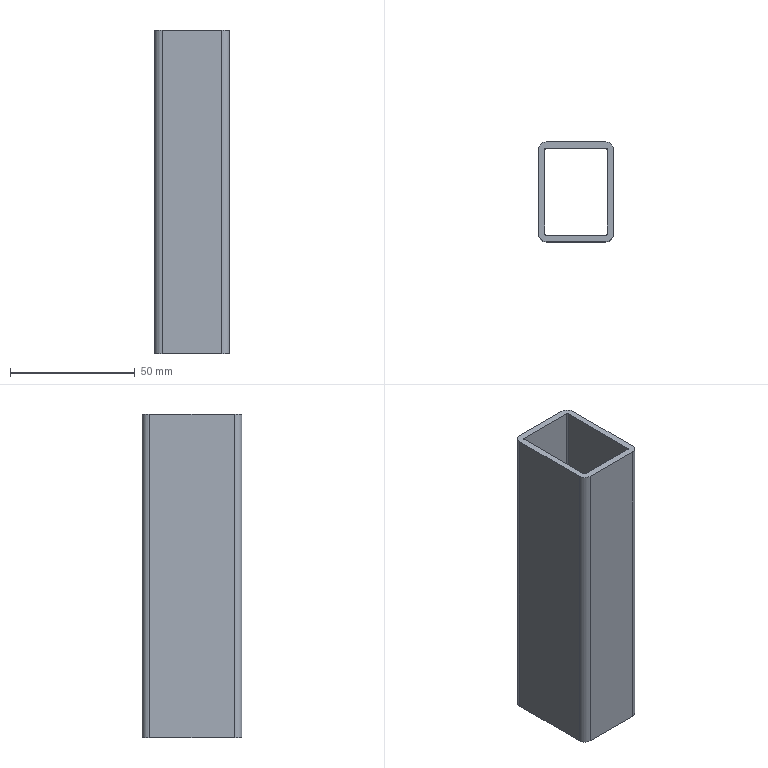Part | SolidWorks | features BaseBody 1 | 1 solid | 18 faces | box 30 x 40 x 130 mm | volume 41274 mm3 | plane 10 | cylinder 8 | commonest cylinder face diameters 1 x4 6 x4
STEP:
#1=CARTESIAN_POINT('',(12.,17.5,-65.));
#2=VERTEX_POINT('',#1);
#3=CARTESIAN_POINT('',(-12.,17.5,-65.));
#4=VERTEX_POINT('',#3);
#5=CARTESIAN_POINT('',(-12.,17.5,-65.));
#6=DIRECTION('',(-1.,0.,0.));
#7=VECTOR('',#6,1000.);
#8=LINE('',#5,#7);
#9=EDGE_CURVE('',#2,#4,#8,.T.);
#10=ORIENTED_EDGE('',*,*,#9,.F.);
#11=CARTESIAN_POINT('',(12.,17.5,65.));
#12=VERTEX_POINT('',#11);
#13=CARTESIAN_POINT('',(12.,17.5,65.));
#14=DIRECTION('',(0.,0.,-1.));
#15=VECTOR('',#14,1000.);
#16=LINE('',#13,#15);
#17=EDGE_CURVE('',#12,#2,#16,.T.);
#18=ORIENTED_EDGE('',*,*,#17,.F.);
#19=CARTESIAN_POINT('',(-12.,17.5,65.));
#20=VERTEX_POINT('',#19);
#21=CARTESIAN_POINT('',(-12.,17.5,65.));
#22=DIRECTION('',(-1.,0.,0.));
#23=VECTOR('',#22,1000.);
#24=LINE('',#21,#23);
#25=EDGE_CURVE('',#12,#20,#24,.T.);
#26=ORIENTED_EDGE('',*,*,#25,.T.);
#27=CARTESIAN_POINT('',(-12.,17.5,65.));
#28=DIRECTION('',(0.,0.,-1.));
#29=VECTOR('',#28,1000.);
#30=LINE('',#27,#29);
#31=EDGE_CURVE('',#20,#4,#30,.T.);
#32=ORIENTED_EDGE('',*,*,#31,.T.);
#33=EDGE_LOOP('',(#10,#18,#26,#32));
#34=FACE_OUTER_BOUND('',#33,.T.);
#35=CARTESIAN_POINT('',(-12.,17.5,65.));
#36=DIRECTION('',(0.,-1.,0.));
#37=DIRECTION('',(0.,0.,-1.));
#38=AXIS2_PLACEMENT_3D('',#35,#36,#37);
#39=PLANE('',#38);
#40=ADVANCED_FACE('',(#34),#39,.T.);
#41=CARTESIAN_POINT('',(12.5,17.,-65.));
#42=VERTEX_POINT('',#41);
#43=CARTESIAN_POINT('',(12.,17.,-65.));
#44=DIRECTION('',(0.,0.,1.));
#45=DIRECTION('',(-1.,0.,0.));
#46=AXIS2_PLACEMENT_3D('',#43,#44,#45);
#47=CIRCLE('',#46,0.5);
#48=EDGE_CURVE('',#42,#2,#47,.T.);
#49=ORIENTED_EDGE('',*,*,#48,.F.);
#50=CARTESIAN_POINT('',(12.5,17.,65.));
#51=VERTEX_POINT('',#50);
#52=CARTESIAN_POINT('',(12.5,17.,65.));
#53=DIRECTION('',(0.,0.,-1.));
#54=VECTOR('',#53,1000.);
#55=LINE('',#52,#54);
#56=EDGE_CURVE('',#51,#42,#55,.T.);
#57=ORIENTED_EDGE('',*,*,#56,.F.);
#58=CARTESIAN_POINT('',(12.,17.,65.));
#59=DIRECTION('',(0.,0.,1.));
#60=DIRECTION('',(-1.,0.,0.));
#61=AXIS2_PLACEMENT_3D('',#58,#59,#60);
#62=CIRCLE('',#61,0.5);
#63=EDGE_CURVE('',#51,#12,#62,.T.);
#64=ORIENTED_EDGE('',*,*,#63,.T.);
#65=ORIENTED_EDGE('',*,*,#17,.T.);
#66=EDGE_LOOP('',(#49,#57,#64,#65));
#67=FACE_OUTER_BOUND('',#66,.T.);
#68=CARTESIAN_POINT('',(12.,17.,65.));
#69=DIRECTION('',(0.,0.,-1.));
#70=DIRECTION('',(-1.,0.,0.));
#71=AXIS2_PLACEMENT_3D('',#68,#69,#70);
#72=CYLINDRICAL_SURFACE('',#71,0.5);
#73=ADVANCED_FACE('',(#67),#72,.F.);
#74=CARTESIAN_POINT('',(12.5,-17.,-65.));
#75=VERTEX_POINT('',#74);
#76=CARTESIAN_POINT('',(12.5,17.,-65.));
#77=DIRECTION('',(0.,1.,0.));
#78=VECTOR('',#77,1000.);
#79=LINE('',#76,#78);
#80=EDGE_CURVE('',#75,#42,#79,.T.);
#81=ORIENTED_EDGE('',*,*,#80,.F.);
#82=CARTESIAN_POINT('',(12.5,-17.,65.));
#83=VERTEX_POINT('',#82);
#84=CARTESIAN_POINT('',(12.5,-17.,65.));
#85=DIRECTION('',(0.,0.,-1.));
#86=VECTOR('',#85,1000.);
#87=LINE('',#84,#86);
#88=EDGE_CURVE('',#83,#75,#87,.T.);
#89=ORIENTED_EDGE('',*,*,#88,.F.);
#90=CARTESIAN_POINT('',(12.5,17.,65.));
#91=DIRECTION('',(0.,1.,0.));
#92=VECTOR('',#91,1000.);
#93=LINE('',#90,#92);
#94=EDGE_CURVE('',#83,#51,#93,.T.);
#95=ORIENTED_EDGE('',*,*,#94,.T.);
#96=ORIENTED_EDGE('',*,*,#56,.T.);
#97=EDGE_LOOP('',(#81,#89,#95,#96));
#98=FACE_OUTER_BOUND('',#97,.T.);
#99=CARTESIAN_POINT('',(12.5,17.,65.));
#100=DIRECTION('',(-1.,0.,0.));
#101=DIRECTION('',(0.,1.,0.));
#102=AXIS2_PLACEMENT_3D('',#99,#100,#101);
#103=PLANE('',#102);
#104=ADVANCED_FACE('',(#98),#103,.T.);
#105=CARTESIAN_POINT('',(12.,-17.5,-65.));
#106=VERTEX_POINT('',#105);
#107=CARTESIAN_POINT('',(12.,-17.,-65.));
#108=DIRECTION('',(0.,0.,1.));
#109=DIRECTION('',(1.,0.,0.));
#110=AXIS2_PLACEMENT_3D('',#107,#108,#109);
#111=CIRCLE('',#110,0.5);
#112=EDGE_CURVE('',#106,#75,#111,.T.);
#113=ORIENTED_EDGE('',*,*,#112,.F.);
#114=CARTESIAN_POINT('',(12.,-17.5,65.));
#115=VERTEX_POINT('',#114);
#116=CARTESIAN_POINT('',(12.,-17.5,65.));
#117=DIRECTION('',(0.,0.,-1.));
#118=VECTOR('',#117,1000.);
#119=LINE('',#116,#118);
#120=EDGE_CURVE('',#115,#106,#119,.T.);
#121=ORIENTED_EDGE('',*,*,#120,.F.);
#122=CARTESIAN_POINT('',(12.,-17.,65.));
#123=DIRECTION('',(0.,0.,1.));
#124=DIRECTION('',(1.,0.,0.));
#125=AXIS2_PLACEMENT_3D('',#122,#123,#124);
#126=CIRCLE('',#125,0.5);
#127=EDGE_CURVE('',#115,#83,#126,.T.);
#128=ORIENTED_EDGE('',*,*,#127,.T.);
#129=ORIENTED_EDGE('',*,*,#88,.T.);
#130=EDGE_LOOP('',(#113,#121,#128,#129));
#131=FACE_OUTER_BOUND('',#130,.T.);
#132=CARTESIAN_POINT('',(12.,-17.,65.));
#133=DIRECTION('',(0.,0.,-1.));
#134=DIRECTION('',(-1.,0.,0.));
#135=AXIS2_PLACEMENT_3D('',#132,#133,#134);
#136=CYLINDRICAL_SURFACE('',#135,0.5);
#137=ADVANCED_FACE('',(#131),#136,.F.);
#138=CARTESIAN_POINT('',(-12.,-17.5,-65.));
#139=VERTEX_POINT('',#138);
#140=CARTESIAN_POINT('',(-12.,-17.5,-65.));
#141=DIRECTION('',(1.,0.,0.));
#142=VECTOR('',#141,1000.);
#143=LINE('',#140,#142);
#144=EDGE_CURVE('',#139,#106,#143,.T.);
#145=ORIENTED_EDGE('',*,*,#144,.F.);
#146=CARTESIAN_POINT('',(-12.,-17.5,65.));
#147=VERTEX_POINT('',#146);
#148=CARTESIAN_POINT('',(-12.,-17.5,65.));
#149=DIRECTION('',(0.,0.,-1.));
#150=VECTOR('',#149,1000.);
#151=LINE('',#148,#150);
#152=EDGE_CURVE('',#147,#139,#151,.T.);
#153=ORIENTED_EDGE('',*,*,#152,.F.);
#154=CARTESIAN_POINT('',(-12.,-17.5,65.));
#155=DIRECTION('',(1.,0.,0.));
#156=VECTOR('',#155,1000.);
#157=LINE('',#154,#156);
#158=EDGE_CURVE('',#147,#115,#157,.T.);
#159=ORIENTED_EDGE('',*,*,#158,.T.);
#160=ORIENTED_EDGE('',*,*,#120,.T.);
#161=EDGE_LOOP('',(#145,#153,#159,#160));
#162=FACE_OUTER_BOUND('',#161,.T.);
#163=CARTESIAN_POINT('',(-12.,-17.5,65.));
#164=DIRECTION('',(0.,1.,0.));
#165=DIRECTION('',(1.,0.,0.));
#166=AXIS2_PLACEMENT_3D('',#163,#164,#165);
#167=PLANE('',#166);
#168=ADVANCED_FACE('',(#162),#167,.T.);
#169=CARTESIAN_POINT('',(-12.5,-17.,-65.));
#170=VERTEX_POINT('',#169);
#171=CARTESIAN_POINT('',(-12.,-17.,-65.));
#172=DIRECTION('',(0.,0.,1.));
#173=DIRECTION('',(1.,0.,0.));
#174=AXIS2_PLACEMENT_3D('',#171,#172,#173);
#175=CIRCLE('',#174,0.5);
#176=EDGE_CURVE('',#170,#139,#175,.T.);
#177=ORIENTED_EDGE('',*,*,#176,.F.);
#178=CARTESIAN_POINT('',(-12.5,-17.,65.));
#179=VERTEX_POINT('',#178);
#180=CARTESIAN_POINT('',(-12.5,-17.,65.));
#181=DIRECTION('',(0.,0.,-1.));
#182=VECTOR('',#181,1000.);
#183=LINE('',#180,#182);
#184=EDGE_CURVE('',#179,#170,#183,.T.);
#185=ORIENTED_EDGE('',*,*,#184,.F.);
#186=CARTESIAN_POINT('',(-12.,-17.,65.));
#187=DIRECTION('',(0.,0.,1.));
#188=DIRECTION('',(1.,0.,0.));
#189=AXIS2_PLACEMENT_3D('',#186,#187,#188);
#190=CIRCLE('',#189,0.5);
#191=EDGE_CURVE('',#179,#147,#190,.T.);
#192=ORIENTED_EDGE('',*,*,#191,.T.);
#193=ORIENTED_EDGE('',*,*,#152,.T.);
#194=EDGE_LOOP('',(#177,#185,#192,#193));
#195=FACE_OUTER_BOUND('',#194,.T.);
#196=CARTESIAN_POINT('',(-12.,-17.,65.));
#197=DIRECTION('',(0.,0.,-1.));
#198=DIRECTION('',(-1.,0.,0.));
#199=AXIS2_PLACEMENT_3D('',#196,#197,#198);
#200=CYLINDRICAL_SURFACE('',#199,0.5);
#201=ADVANCED_FACE('',(#195),#200,.F.);
#202=CARTESIAN_POINT('',(-12.5,17.,-65.));
#203=VERTEX_POINT('',#202);
#204=CARTESIAN_POINT('',(-12.5,17.,-65.));
#205=DIRECTION('',(0.,-1.,0.));
#206=VECTOR('',#205,1000.);
#207=LINE('',#204,#206);
#208=EDGE_CURVE('',#203,#170,#207,.T.);
#209=ORIENTED_EDGE('',*,*,#208,.F.);
#210=CARTESIAN_POINT('',(-12.5,17.,65.));
#211=VERTEX_POINT('',#210);
#212=CARTESIAN_POINT('',(-12.5,17.,65.));
#213=DIRECTION('',(0.,0.,-1.));
#214=VECTOR('',#213,1000.);
#215=LINE('',#212,#214);
#216=EDGE_CURVE('',#211,#203,#215,.T.);
#217=ORIENTED_EDGE('',*,*,#216,.F.);
#218=CARTESIAN_POINT('',(-12.5,17.,65.));
#219=DIRECTION('',(0.,-1.,0.));
#220=VECTOR('',#219,1000.);
#221=LINE('',#218,#220);
#222=EDGE_CURVE('',#211,#179,#221,.T.);
#223=ORIENTED_EDGE('',*,*,#222,.T.);
#224=ORIENTED_EDGE('',*,*,#184,.T.);
#225=EDGE_LOOP('',(#209,#217,#223,#224));
#226=FACE_OUTER_BOUND('',#225,.T.);
#227=CARTESIAN_POINT('',(-12.5,17.,65.));
#228=DIRECTION('',(1.,0.,0.));
#229=DIRECTION('',(0.,1.,0.));
#230=AXIS2_PLACEMENT_3D('',#227,#228,#229);
#231=PLANE('',#230);
#232=ADVANCED_FACE('',(#226),#231,.T.);
#233=CARTESIAN_POINT('',(-12.,17.,-65.));
#234=DIRECTION('',(0.,0.,1.));
#235=DIRECTION('',(1.,0.,0.));
#236=AXIS2_PLACEMENT_3D('',#233,#234,#235);
#237=CIRCLE('',#236,0.5);
#238=EDGE_CURVE('',#4,#203,#237,.T.);
#239=ORIENTED_EDGE('',*,*,#238,.F.);
#240=ORIENTED_EDGE('',*,*,#31,.F.);
#241=CARTESIAN_POINT('',(-12.,17.,65.));
#242=DIRECTION('',(0.,0.,1.));
#243=DIRECTION('',(1.,0.,0.));
#244=AXIS2_PLACEMENT_3D('',#241,#242,#243);
#245=CIRCLE('',#244,0.5);
#246=EDGE_CURVE('',#20,#211,#245,.T.);
#247=ORIENTED_EDGE('',*,*,#246,.T.);
#248=ORIENTED_EDGE('',*,*,#216,.T.);
#249=EDGE_LOOP('',(#239,#240,#247,#248));
#250=FACE_OUTER_BOUND('',#249,.T.);
#251=CARTESIAN_POINT('',(-12.,17.,65.));
#252=DIRECTION('',(0.,0.,-1.));
#253=DIRECTION('',(-1.,0.,0.));
#254=AXIS2_PLACEMENT_3D('',#251,#252,#253);
#255=CYLINDRICAL_SURFACE('',#254,0.5);
#256=ADVANCED_FACE('',(#250),#255,.F.);
#257=CARTESIAN_POINT('',(-15.,17.,-65.));
#258=VERTEX_POINT('',#257);
#259=CARTESIAN_POINT('',(-15.,-17.,-65.));
#260=VERTEX_POINT('',#259);
#261=CARTESIAN_POINT('',(-15.,17.,-65.));
#262=DIRECTION('',(0.,-1.,0.));
#263=VECTOR('',#262,1000.);
#264=LINE('',#261,#263);
#265=EDGE_CURVE('',#258,#260,#264,.T.);
#266=ORIENTED_EDGE('',*,*,#265,.T.);
#267=CARTESIAN_POINT('',(-15.,-17.,65.));
#268=VERTEX_POINT('',#267);
#269=CARTESIAN_POINT('',(-15.,-17.,65.));
#270=DIRECTION('',(0.,0.,-1.));
#271=VECTOR('',#270,1000.);
#272=LINE('',#269,#271);
#273=EDGE_CURVE('',#268,#260,#272,.T.);
#274=ORIENTED_EDGE('',*,*,#273,.F.);
#275=CARTESIAN_POINT('',(-15.,17.,65.));
#276=VERTEX_POINT('',#275);
#277=CARTESIAN_POINT('',(-15.,17.,65.));
#278=DIRECTION('',(0.,-1.,0.));
#279=VECTOR('',#278,1000.);
#280=LINE('',#277,#279);
#281=EDGE_CURVE('',#276,#268,#280,.T.);
#282=ORIENTED_EDGE('',*,*,#281,.F.);
#283=CARTESIAN_POINT('',(-15.,17.,65.));
#284=DIRECTION('',(0.,0.,-1.));
#285=VECTOR('',#284,1000.);
#286=LINE('',#283,#285);
#287=EDGE_CURVE('',#276,#258,#286,.T.);
#288=ORIENTED_EDGE('',*,*,#287,.T.);
#289=EDGE_LOOP('',(#266,#274,#282,#288));
#290=FACE_OUTER_BOUND('',#289,.T.);
#291=CARTESIAN_POINT('',(-15.,17.,65.));
#292=DIRECTION('',(1.,0.,0.));
#293=DIRECTION('',(0.,1.,0.));
#294=AXIS2_PLACEMENT_3D('',#291,#292,#293);
#295=PLANE('',#294);
#296=ADVANCED_FACE('',(#290),#295,.F.);
#297=CARTESIAN_POINT('',(-12.,20.,-65.));
#298=VERTEX_POINT('',#297);
#299=CARTESIAN_POINT('',(-12.,17.,-65.));
#300=DIRECTION('',(0.,0.,1.));
#301=DIRECTION('',(1.,0.,0.));
#302=AXIS2_PLACEMENT_3D('',#299,#300,#301);
#303=CIRCLE('',#302,3.);
#304=EDGE_CURVE('',#298,#258,#303,.T.);
#305=ORIENTED_EDGE('',*,*,#304,.T.);
#306=ORIENTED_EDGE('',*,*,#287,.F.);
#307=CARTESIAN_POINT('',(-12.,20.,65.));
#308=VERTEX_POINT('',#307);
#309=CARTESIAN_POINT('',(-12.,17.,65.));
#310=DIRECTION('',(0.,0.,1.));
#311=DIRECTION('',(1.,0.,0.));
#312=AXIS2_PLACEMENT_3D('',#309,#310,#311);
#313=CIRCLE('',#312,3.);
#314=EDGE_CURVE('',#308,#276,#313,.T.);
#315=ORIENTED_EDGE('',*,*,#314,.F.);
#316=CARTESIAN_POINT('',(-12.,20.,65.));
#317=DIRECTION('',(0.,0.,-1.));
#318=VECTOR('',#317,1000.);
#319=LINE('',#316,#318);
#320=EDGE_CURVE('',#308,#298,#319,.T.);
#321=ORIENTED_EDGE('',*,*,#320,.T.);
#322=EDGE_LOOP('',(#305,#306,#315,#321));
#323=FACE_OUTER_BOUND('',#322,.T.);
#324=CARTESIAN_POINT('',(-12.,17.,65.));
#325=DIRECTION('',(0.,0.,-1.));
#326=DIRECTION('',(-1.,0.,0.));
#327=AXIS2_PLACEMENT_3D('',#324,#325,#326);
#328=CYLINDRICAL_SURFACE('',#327,3.);
#329=ADVANCED_FACE('',(#323),#328,.T.);
#330=CARTESIAN_POINT('',(12.,20.,-65.));
#331=VERTEX_POINT('',#330);
#332=CARTESIAN_POINT('',(-12.,20.,-65.));
#333=DIRECTION('',(-1.,0.,0.));
#334=VECTOR('',#333,1000.);
#335=LINE('',#332,#334);
#336=EDGE_CURVE('',#331,#298,#335,.T.);
#337=ORIENTED_EDGE('',*,*,#336,.T.);
#338=ORIENTED_EDGE('',*,*,#320,.F.);
#339=CARTESIAN_POINT('',(12.,20.,65.));
#340=VERTEX_POINT('',#339);
#341=CARTESIAN_POINT('',(-12.,20.,65.));
#342=DIRECTION('',(-1.,0.,0.));
#343=VECTOR('',#342,1000.);
#344=LINE('',#341,#343);
#345=EDGE_CURVE('',#340,#308,#344,.T.);
#346=ORIENTED_EDGE('',*,*,#345,.F.);
#347=CARTESIAN_POINT('',(12.,20.,65.));
#348=DIRECTION('',(0.,0.,-1.));
#349=VECTOR('',#348,1000.);
#350=LINE('',#347,#349);
#351=EDGE_CURVE('',#340,#331,#350,.T.);
#352=ORIENTED_EDGE('',*,*,#351,.T.);
#353=EDGE_LOOP('',(#337,#338,#346,#352));
#354=FACE_OUTER_BOUND('',#353,.T.);
#355=CARTESIAN_POINT('',(-12.,20.,65.));
#356=DIRECTION('',(0.,-1.,0.));
#357=DIRECTION('',(0.,0.,-1.));
#358=AXIS2_PLACEMENT_3D('',#355,#356,#357);
#359=PLANE('',#358);
#360=ADVANCED_FACE('',(#354),#359,.F.);
#361=CARTESIAN_POINT('',(15.,17.,-65.));
#362=VERTEX_POINT('',#361);
#363=CARTESIAN_POINT('',(12.,17.,-65.));
#364=DIRECTION('',(0.,0.,1.));
#365=DIRECTION('',(-1.,0.,0.));
#366=AXIS2_PLACEMENT_3D('',#363,#364,#365);
#367=CIRCLE('',#366,3.);
#368=EDGE_CURVE('',#362,#331,#367,.T.);
#369=ORIENTED_EDGE('',*,*,#368,.T.);
#370=ORIENTED_EDGE('',*,*,#351,.F.);
#371=CARTESIAN_POINT('',(15.,17.,65.));
#372=VERTEX_POINT('',#371);
#373=CARTESIAN_POINT('',(12.,17.,65.));
#374=DIRECTION('',(0.,0.,1.));
#375=DIRECTION('',(-1.,0.,0.));
#376=AXIS2_PLACEMENT_3D('',#373,#374,#375);
#377=CIRCLE('',#376,3.);
#378=EDGE_CURVE('',#372,#340,#377,.T.);
#379=ORIENTED_EDGE('',*,*,#378,.F.);
#380=CARTESIAN_POINT('',(15.,17.,65.));
#381=DIRECTION('',(0.,0.,-1.));
#382=VECTOR('',#381,1000.);
#383=LINE('',#380,#382);
#384=EDGE_CURVE('',#372,#362,#383,.T.);
#385=ORIENTED_EDGE('',*,*,#384,.T.);
#386=EDGE_LOOP('',(#369,#370,#379,#385));
#387=FACE_OUTER_BOUND('',#386,.T.);
#388=CARTESIAN_POINT('',(12.,17.,65.));
#389=DIRECTION('',(0.,0.,-1.));
#390=DIRECTION('',(-1.,0.,0.));
#391=AXIS2_PLACEMENT_3D('',#388,#389,#390);
#392=CYLINDRICAL_SURFACE('',#391,3.);
#393=ADVANCED_FACE('',(#387),#392,.T.);
#394=CARTESIAN_POINT('',(15.,-17.,-65.));
#395=VERTEX_POINT('',#394);
#396=CARTESIAN_POINT('',(15.,17.,-65.));
#397=DIRECTION('',(0.,1.,0.));
#398=VECTOR('',#397,1000.);
#399=LINE('',#396,#398);
#400=EDGE_CURVE('',#395,#362,#399,.T.);
#401=ORIENTED_EDGE('',*,*,#400,.T.);
#402=ORIENTED_EDGE('',*,*,#384,.F.);
#403=CARTESIAN_POINT('',(15.,-17.,65.));
#404=VERTEX_POINT('',#403);
#405=CARTESIAN_POINT('',(15.,17.,65.));
#406=DIRECTION('',(0.,1.,0.));
#407=VECTOR('',#406,1000.);
#408=LINE('',#405,#407);
#409=EDGE_CURVE('',#404,#372,#408,.T.);
#410=ORIENTED_EDGE('',*,*,#409,.F.);
#411=CARTESIAN_POINT('',(15.,-17.,65.));
#412=DIRECTION('',(0.,0.,-1.));
#413=VECTOR('',#412,1000.);
#414=LINE('',#411,#413);
#415=EDGE_CURVE('',#404,#395,#414,.T.);
#416=ORIENTED_EDGE('',*,*,#415,.T.);
#417=EDGE_LOOP('',(#401,#402,#410,#416));
#418=FACE_OUTER_BOUND('',#417,.T.);
#419=CARTESIAN_POINT('',(15.,17.,65.));
#420=DIRECTION('',(-1.,0.,0.));
#421=DIRECTION('',(0.,1.,0.));
#422=AXIS2_PLACEMENT_3D('',#419,#420,#421);
#423=PLANE('',#422);
#424=ADVANCED_FACE('',(#418),#423,.F.);
#425=CARTESIAN_POINT('',(12.,-20.,-65.));
#426=VERTEX_POINT('',#425);
#427=CARTESIAN_POINT('',(12.,-17.,-65.));
#428=DIRECTION('',(0.,0.,1.));
#429=DIRECTION('',(1.,0.,0.));
#430=AXIS2_PLACEMENT_3D('',#427,#428,#429);
#431=CIRCLE('',#430,3.);
#432=EDGE_CURVE('',#426,#395,#431,.T.);
#433=ORIENTED_EDGE('',*,*,#432,.T.);
#434=ORIENTED_EDGE('',*,*,#415,.F.);
#435=CARTESIAN_POINT('',(12.,-20.,65.));
#436=VERTEX_POINT('',#435);
#437=CARTESIAN_POINT('',(12.,-17.,65.));
#438=DIRECTION('',(0.,0.,1.));
#439=DIRECTION('',(1.,0.,0.));
#440=AXIS2_PLACEMENT_3D('',#437,#438,#439);
#441=CIRCLE('',#440,3.);
#442=EDGE_CURVE('',#436,#404,#441,.T.);
#443=ORIENTED_EDGE('',*,*,#442,.F.);
#444=CARTESIAN_POINT('',(12.,-20.,65.));
#445=DIRECTION('',(0.,0.,-1.));
#446=VECTOR('',#445,1000.);
#447=LINE('',#444,#446);
#448=EDGE_CURVE('',#436,#426,#447,.T.);
#449=ORIENTED_EDGE('',*,*,#448,.T.);
#450=EDGE_LOOP('',(#433,#434,#443,#449));
#451=FACE_OUTER_BOUND('',#450,.T.);
#452=CARTESIAN_POINT('',(12.,-17.,65.));
#453=DIRECTION('',(0.,0.,-1.));
#454=DIRECTION('',(-1.,0.,0.));
#455=AXIS2_PLACEMENT_3D('',#452,#453,#454);
#456=CYLINDRICAL_SURFACE('',#455,3.);
#457=ADVANCED_FACE('',(#451),#456,.T.);
#458=CARTESIAN_POINT('',(-12.,-20.,-65.));
#459=VERTEX_POINT('',#458);
#460=CARTESIAN_POINT('',(-12.,-20.,-65.));
#461=DIRECTION('',(1.,0.,0.));
#462=VECTOR('',#461,1000.);
#463=LINE('',#460,#462);
#464=EDGE_CURVE('',#459,#426,#463,.T.);
#465=ORIENTED_EDGE('',*,*,#464,.T.);
#466=ORIENTED_EDGE('',*,*,#448,.F.);
#467=CARTESIAN_POINT('',(-12.,-20.,65.));
#468=VERTEX_POINT('',#467);
#469=CARTESIAN_POINT('',(-12.,-20.,65.));
#470=DIRECTION('',(1.,0.,0.));
#471=VECTOR('',#470,1000.);
#472=LINE('',#469,#471);
#473=EDGE_CURVE('',#468,#436,#472,.T.);
#474=ORIENTED_EDGE('',*,*,#473,.F.);
#475=CARTESIAN_POINT('',(-12.,-20.,65.));
#476=DIRECTION('',(0.,0.,-1.));
#477=VECTOR('',#476,1000.);
#478=LINE('',#475,#477);
#479=EDGE_CURVE('',#468,#459,#478,.T.);
#480=ORIENTED_EDGE('',*,*,#479,.T.);
#481=EDGE_LOOP('',(#465,#466,#474,#480));
#482=FACE_OUTER_BOUND('',#481,.T.);
#483=CARTESIAN_POINT('',(-12.,-20.,65.));
#484=DIRECTION('',(0.,1.,0.));
#485=DIRECTION('',(1.,0.,0.));
#486=AXIS2_PLACEMENT_3D('',#483,#484,#485);
#487=PLANE('',#486);
#488=ADVANCED_FACE('',(#482),#487,.F.);
#489=CARTESIAN_POINT('',(-12.,-17.,-65.));
#490=DIRECTION('',(0.,0.,1.));
#491=DIRECTION('',(1.,0.,0.));
#492=AXIS2_PLACEMENT_3D('',#489,#490,#491);
#493=CIRCLE('',#492,3.);
#494=EDGE_CURVE('',#260,#459,#493,.T.);
#495=ORIENTED_EDGE('',*,*,#494,.T.);
#496=ORIENTED_EDGE('',*,*,#479,.F.);
#497=CARTESIAN_POINT('',(-12.,-17.,65.));
#498=DIRECTION('',(0.,0.,1.));
#499=DIRECTION('',(1.,0.,0.));
#500=AXIS2_PLACEMENT_3D('',#497,#498,#499);
#501=CIRCLE('',#500,3.);
#502=EDGE_CURVE('',#268,#468,#501,.T.);
#503=ORIENTED_EDGE('',*,*,#502,.F.);
#504=ORIENTED_EDGE('',*,*,#273,.T.);
#505=EDGE_LOOP('',(#495,#496,#503,#504));
#506=FACE_OUTER_BOUND('',#505,.T.);
#507=CARTESIAN_POINT('',(-12.,-17.,65.));
#508=DIRECTION('',(0.,0.,-1.));
#509=DIRECTION('',(-1.,0.,0.));
#510=AXIS2_PLACEMENT_3D('',#507,#508,#509);
#511=CYLINDRICAL_SURFACE('',#510,3.);
#512=ADVANCED_FACE('',(#506),#511,.T.);
#513=ORIENTED_EDGE('',*,*,#238,.T.);
#514=ORIENTED_EDGE('',*,*,#208,.T.);
#515=ORIENTED_EDGE('',*,*,#176,.T.);
#516=ORIENTED_EDGE('',*,*,#144,.T.);
#517=ORIENTED_EDGE('',*,*,#112,.T.);
#518=ORIENTED_EDGE('',*,*,#80,.T.);
#519=ORIENTED_EDGE('',*,*,#48,.T.);
#520=ORIENTED_EDGE('',*,*,#9,.T.);
#521=EDGE_LOOP('',(#513,#514,#515,#516,#517,#518,#519,#520));
#522=FACE_BOUND('',#521,.T.);
#523=ORIENTED_EDGE('',*,*,#494,.F.);
#524=ORIENTED_EDGE('',*,*,#265,.F.);
#525=ORIENTED_EDGE('',*,*,#304,.F.);
#526=ORIENTED_EDGE('',*,*,#336,.F.);
#527=ORIENTED_EDGE('',*,*,#368,.F.);
#528=ORIENTED_EDGE('',*,*,#400,.F.);
#529=ORIENTED_EDGE('',*,*,#432,.F.);
#530=ORIENTED_EDGE('',*,*,#464,.F.);
#531=EDGE_LOOP('',(#523,#524,#525,#526,#527,#528,#529,#530));
#532=FACE_OUTER_BOUND('',#531,.T.);
#533=CARTESIAN_POINT('',(-12.,-17.,-65.));
#534=DIRECTION('',(0.,0.,1.));
#535=DIRECTION('',(1.,0.,0.));
#536=AXIS2_PLACEMENT_3D('',#533,#534,#535);
#537=PLANE('',#536);
#538=ADVANCED_FACE('',(#522,#532),#537,.F.);
#539=ORIENTED_EDGE('',*,*,#222,.F.);
#540=ORIENTED_EDGE('',*,*,#246,.F.);
#541=ORIENTED_EDGE('',*,*,#25,.F.);
#542=ORIENTED_EDGE('',*,*,#63,.F.);
#543=ORIENTED_EDGE('',*,*,#94,.F.);
#544=ORIENTED_EDGE('',*,*,#127,.F.);
#545=ORIENTED_EDGE('',*,*,#158,.F.);
#546=ORIENTED_EDGE('',*,*,#191,.F.);
#547=EDGE_LOOP('',(#539,#540,#541,#542,#543,#544,#545,#546));
#548=FACE_BOUND('',#547,.T.);
#549=ORIENTED_EDGE('',*,*,#502,.T.);
#550=ORIENTED_EDGE('',*,*,#473,.T.);
#551=ORIENTED_EDGE('',*,*,#442,.T.);
#552=ORIENTED_EDGE('',*,*,#409,.T.);
#553=ORIENTED_EDGE('',*,*,#378,.T.);
#554=ORIENTED_EDGE('',*,*,#345,.T.);
#555=ORIENTED_EDGE('',*,*,#314,.T.);
#556=ORIENTED_EDGE('',*,*,#281,.T.);
#557=EDGE_LOOP('',(#549,#550,#551,#552,#553,#554,#555,#556));
#558=FACE_OUTER_BOUND('',#557,.T.);
#559=CARTESIAN_POINT('',(-12.,-17.,65.));
#560=DIRECTION('',(0.,0.,1.));
#561=DIRECTION('',(1.,0.,0.));
#562=AXIS2_PLACEMENT_3D('',#559,#560,#561);
#563=PLANE('',#562);
#564=ADVANCED_FACE('',(#548,#558),#563,.T.);
#565=CLOSED_SHELL('',(#40,#73,#104,#137,#168,#201,#232,#256,#296,#329,#360,#393,#424,#457,#488,#512,#538,#564));
#566=MANIFOLD_SOLID_BREP('',#565);
#567=CARTESIAN_POINT('',(0.,0.,0.));
#568=DIRECTION('',(0.,0.,1.));
#569=DIRECTION('',(1.,0.,0.));
#570=AXIS2_PLACEMENT_3D('',#567,#568,#569);
#571=(LENGTH_UNIT()NAMED_UNIT(*)SI_UNIT(.MILLI.,.METRE.));
#572=UNCERTAINTY_MEASURE_WITH_UNIT(LENGTH_MEASURE(0.00001),#571,'','');
#573=(NAMED_UNIT(*)PLANE_ANGLE_UNIT()SI_UNIT($,.RADIAN.));
#574=(NAMED_UNIT(*)SI_UNIT($,.STERADIAN.)SOLID_ANGLE_UNIT());
#575=(GEOMETRIC_REPRESENTATION_CONTEXT(3)GLOBAL_UNCERTAINTY_ASSIGNED_CONTEXT((#572))GLOBAL_UNIT_ASSIGNED_CONTEXT((#571,#573,#574))REPRESENTATION_CONTEXT('',''));
#576=ADVANCED_BREP_SHAPE_REPRESENTATION('',(#566,#570),#575);